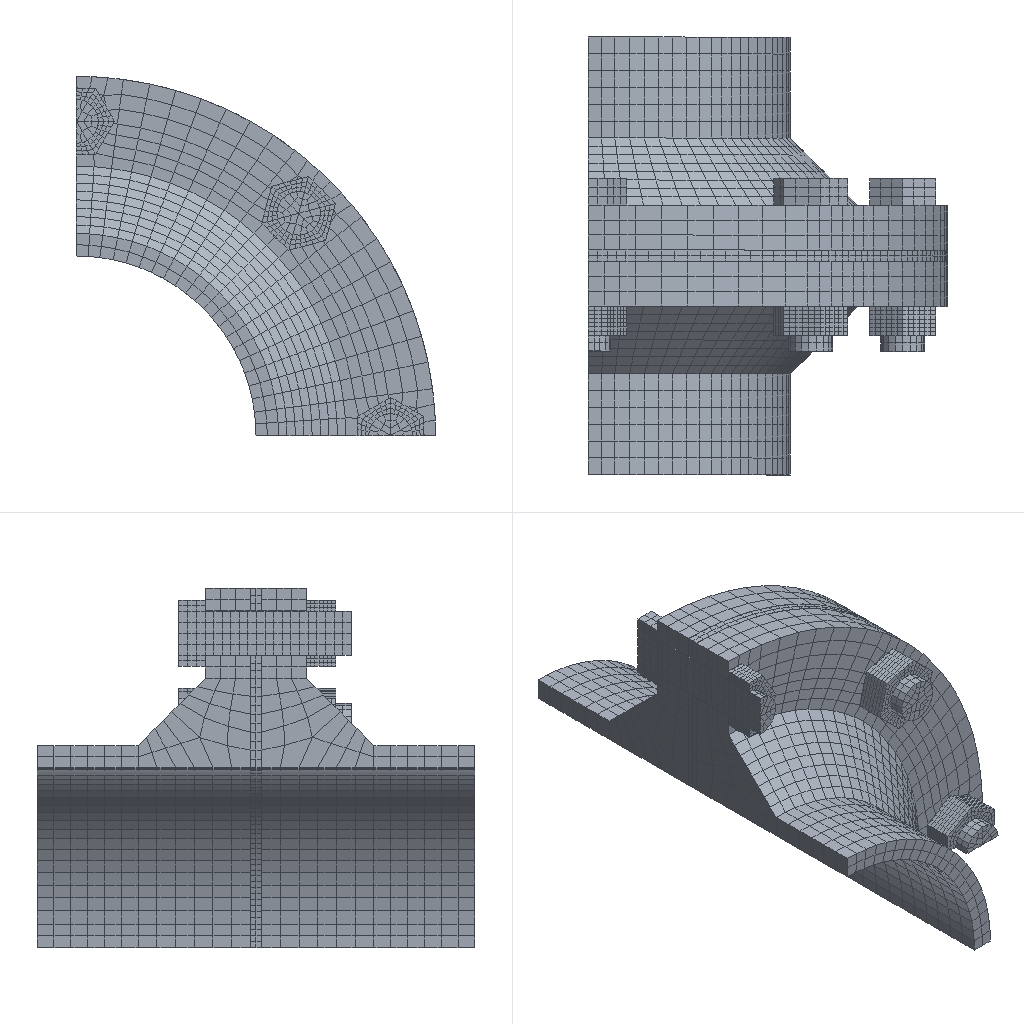Simulation study | abaqus
Set-up summary:
category,name,step,type,value,unit,region
solver,abaqus,,Abaqus/CAE 2024
units,mm-mN-s-kg (kPa) or mm-kg-s,,inferred,E=1.4935e+07 density=
analysis,Tighten bolts,,static,nlgeom=True; time_period=1
mesh,nodes,,,11472
mesh,elements,,,7304
element_type,C3D8R,,,5496
element_type,C3D8H,,,1808
material,brass,,E,1.4935e+07
material,brass,,nu,0.3
material,brass,,yield,28000
material,brass,,behaviors,plastic
material,rubber,,behaviors,hyperelastic
material,steel,,E,3e+07
material,steel,,nu,0.3
material,steel,,yield,52000
material,steel,,behaviors,plastic
section,steel,,solid section,,,all
section,brass,,solid section,,,all
section,rubber,,solid section,,,all
section,steel,,solid section,,,all
section,steel,,solid section,,,all
section,steel,,solid section,,,all
load,Load-1,Tighten bolts,concentrated force,"200 [dir=(1, 0, 0)]",,_Load-1_blrn_
load,Load-2,Tighten bolts,concentrated force,"100 [dir=(1, 0, 0)]",,_Load-2_blrn_
load,Load-3,Tighten bolts,concentrated force,"100 [dir=(1, 0, 0)]",,_Load-3_blrn_
bc,Bottom,Tighten bolts,fixed,[dofs=y],,Bottom
bc,Csymm-x,Tighten bolts,fixed,[dofs=x],,Csymm-x
bc,Csymm-z,Tighten bolts,fixed,[dofs=z],,Csymm-z
contact,CP-1-HalfBolt-1-HalfNut-1,initial,tie,,,CP-1-HalfNut-1 / CP-1-HalfBolt-1
contact,CP-2-Bolt-1-nut-1,initial,tie,,,CP-2-nut-1 / CP-2-Bolt-1
contact,CP-3-HalfBolt-2-HalfNut-2,initial,tie,,,CP-3-HalfNut-2 / CP-3-HalfBolt-2
contact,CP-1-botFlange-Gasket-1,initial,contact pair surface to surface,interaction=Friction-0p4; friction=0.4; behavior=hard,,CP-1-Gasket-1 / CP-1-botFlange
contact,CP-2-botFlange-Bolt-1,initial,contact pair surface to surface,interaction=Friction-0p1; friction=0.1; behavior=hard,,CP-3-Bolt-1 / CP-2-botFlange
contact,CP-3-botFlange-nut-1,initial,contact pair surface to surface,interaction=Friction-0p1; friction=0.1; behavior=hard,,CP-3-nut-1 / CP-3-botFlange
contact,CP-4-botFlange-HalfBolt-1,initial,contact pair surface to surface,interaction=Friction-0p1; friction=0.1; behavior=hard,,CP-4-HalfBolt-1 / CP-4-botFlange
contact,CP-5-botFlange-HalfNut-1,initial,contact pair surface to surface,interaction=Friction-0p1; friction=0.1; behavior=hard,,CP-5-HalfNut-1 / CP-5-botFlange
contact,CP-6-botFlange-HalfBolt-2,initial,contact pair surface to surface,interaction=Friction-0p1; friction=0.1; behavior=hard,,CP-6-HalfBolt-2 / CP-6-botFlange
contact,CP-7-botFlange-HalfNut-2,initial,contact pair surface to surface,interaction=Friction-0p1; friction=0.1; behavior=hard,,CP-7-HalfNut-2 / CP-7-botFlange
contact,CP-8-topFlange-Gasket-1,initial,contact pair surface to surface,interaction=Friction-0p4; friction=0.4; behavior=hard,,CP-8-Gasket-1 / CP-8-topFlange
contact,CP-9-topFlange-Bolt-1,initial,contact pair surface to surface,interaction=Friction-0p1; friction=0.1; behavior=hard,,CP-9-Bolt-1 / CP-9-topFlange
contact,CP-10-topFlange-Bolt-1,initial,contact pair surface to surface,interaction=Friction-0p1; friction=0.1; behavior=hard,,CP-10-Bolt-1 / CP-10-topFlange
contact,CP-11-topFlange-HalfBolt-1,initial,contact pair surface to surface,interaction=Friction-0p1; friction=0.1; behavior=hard,,CP-11-HalfBolt-1 / CP-11-topFlange
contact,CP-12-topFlange-HalfBolt-1,initial,contact pair surface to surface,interaction=Friction-0p1; friction=0.1; behavior=hard,,CP-12-HalfBolt-1 / CP-12-topFlange
contact,CP-13-topFlange-HalfBolt-2,initial,contact pair surface to surface,interaction=Friction-0p1; friction=0.1; behavior=hard,,CP-13-HalfBolt-2 / CP-13-topFlange
contact,CP-14-topFlange-HalfBolt-2,initial,contact pair surface to surface,interaction=Friction-0p1; friction=0.1; behavior=hard,,CP-14-HalfBolt-2 / CP-14-topFlange
contact,CP-15-Bolt-1-Gasket-1,initial,contact pair surface to surface,interaction=Friction-0p4; friction=0.4; behavior=hard,,CP-15-Gasket-1 / CP-15-Bolt-1
contact,CP-16-HalfBolt-1-Gasket-1,initial,contact pair surface to surface,interaction=Friction-0p4; friction=0.4; behavior=hard,,CP-16-Gasket-1 / CP-16-HalfBolt-1
contact,CP-17-HalfBolt-2-Gasket-1,initial,contact pair surface to surface,interaction=Friction-0p4; friction=0.4; behavior=hard,,CP-17-Gasket-1 / CP-17-HalfBolt-2
Abaqus input file, long lists of numbers shortened, first 294 of 1956 lines:
*Heading
** Job name: deck Model name: Model-1
** Generated by: Abaqus/CAE 2024
*Preprint, echo=NO, model=NO, history=NO, contact=NO
**
** PARTS
**
*Part, name=bolt
*Node
      1, -1.5239944e-10,  0.85, -4.02707534e-10
      2,  0.1225,  0.85,  0.2122
** (982 more lines like these left out)
*Element, type=C3D8R
 1, 318,  55, 294, 770,  41,   1,  42, 292
 2, 770, 294, 295, 763, 292,  42,  43, 293
** (706 more lines like these left out)
*Nset, nset=all, generate
   1,  984,    1
*Elset, elset=all, generate
   1,  708,    1
*Elset, elset=_boltLoad_S2, internal
   1,   2,  13,  19,  20,  66,  67,  78,  84,  85, 131, 132, 143, 149, 150, 196
 202, 203, 214, 215, 261, 262, 273, 279, 280, 504
*Elset, elset=_boltLoad_S4, internal
 482, 489
*Elset, elset=_boltLoad_S3, internal
 490, 497
*Surface, type=ELEMENT, name=boltLoad
_boltLoad_S2, S2
_boltLoad_S4, S4
_boltLoad_S3, S3
** Section: bolt
*Solid Section, elset=all, material=steel
1.,
*End Part
**
*Part, name=flange
*Node
      1,           2.,  0.5244,           0.
      2,   1.983,  0.5244,   0.2611
** (1981 more lines like these left out)
*Element, type=C3D8R
 1,  634,  635, 1561, 1560,   93,   94,  629,  628
 2,  635,  636, 1562, 1561,   94,   95,  630,  629
** (1256 more lines like these left out)
*Nset, nset=all, generate
    1,  1983,     1
*Elset, elset=all, generate
    1,  1258,     1
** Section: flange
*Solid Section, elset=all, material=brass
1.,
*End Part
**
*Part, name=gasket
*Node
      1,   3.47,  0.4568,        0.125
      2,   3.47,  0.4568,           0.
** (2965 more lines like these left out)
*Element, type=C3D8H
 1,  716,   74,  706, 2319,   71,    1,   73,  704
 2, 2319,  706,  707, 2316,  704,   73,   72,  705
** (1806 more lines like these left out)
*Nset, nset=all, generate
    1,  2967,     1
*Elset, elset=all, generate
    1,  1808,     1
** Section: gasket
*Solid Section, elset=all, material=rubber
1.,
*End Part
**
*Part, name=halfBolt
*Node
      1, -6.66499911e-11,   1.225, -1.78729587e-10
      2, -0.2122,   1.225, -0.1225
** (590 more lines like these left out)
*Element, type=C3D8R
 1, 221,  37, 218, 480,  35,   1,  36, 217
 2, 222,  38, 219, 479, 221,  37, 218, 480
** (378 more lines like these left out)
*Nset, nset=all, generate
   1,  592,    1
*Elset, elset=all, generate
   1,  380,    1
*Elset, elset=_boltLoad_S4, internal
  37,  51, 130, 195, 202
*Elset, elset=_boltLoad_S3, internal
  38, 131, 175, 182
*Elset, elset=_boltLoad_S2, internal
 138, 203, 250, 251, 262, 263, 274
*Surface, type=ELEMENT, name=boltLoad
_boltLoad_S4, S4
_boltLoad_S3, S3
_boltLoad_S2, S2
** Section: bolt
*Solid Section, elset=all, material=steel
1.,
*End Part
**
*Part, name=halfNut
*Node
      1, -0.2125, -0.3681,  0.325
      2, -0.425,           0.,  0.325
** (606 more lines like these left out)
*Element, type=C3D8R
  1,  67, 241, 441, 217,   1,  21, 157,  42
  2, 241, 242, 442, 441,  21,  22, 158, 157
** (376 more lines like these left out)
*Nset, nset=all, generate
   1,  608,    1
*Elset, elset=all, generate
   1,  378,    1
** Section: bolt
*Solid Section, elset=all, material=steel
1.,
*End Part
**
*Part, name=nut
*Node
      1,  0.425,           0.,  0.325
      2,  0.2125, -0.3681,  0.325
** (1150 more lines like these left out)
*Element, type=C3D8R
  1,  72, 325, 793, 301,   1,  25, 241,  46
  2, 325, 326, 794, 793,  25,  26, 242, 241
** (754 more lines like these left out)
*Nset, nset=all, generate
    1,  1152,     1
*Elset, elset=all, generate
   1,  756,    1
** Section: bolt
*Solid Section, elset=all, material=steel
1.,
*End Part
**
**
** ASSEMBLY
**
*Assembly, name=Assembly
**
*Instance, name=botFlange, part=flange
*End Instance
**
*Instance, name=topFlange, part=flange
          0.,     3.674,           0.
          0.,     3.674,           0., 0.7071,     3.674, 0.7071,         180.
*End Instance
**
*Instance, name=Gasket-1, part=gasket
          0.,     1.774, -8.99865743746394e-13
          0.,     1.774, -8.99865743746394e-13, 0.5774, 2.352, 0.5774,         240.
*End Instance
**
*Instance, name=Bolt-1, part=bolt
2.475,     1.174, 2.475
2.475,     1.174, 2.475, 2.475, 0.1744, 2.475, 15.
*End Instance
**
*Instance, name=nut-1, part=nut
2.475,     1.274, 2.475
2.475,     1.274, 2.475, 3.458, 1.145, 2.604, 90.976
*End Instance
**
*Instance, name=HalfBolt-1, part=halfBolt
          0.,     1.174,          3.5
          0.,     1.174,          3.5,           0.,     0.1744,          3.5, 60.
*End Instance
**
*Instance, name=HalfNut-1, part=halfNut
1.63712270681787e-11,     1.274,          3.5
1.63712270681787e-11,     1.274,          3.5, 1.8118469336612e-11, 1.981, 2.793, 180.
*End Instance
**
*Instance, name=HalfBolt-2, part=halfBolt
         3.5,     1.174, 2.45732323378434e-11
         3.5,     1.174, 2.45732323378434e-11,          3.5, 2.174, 2.45732323378434e-11, 210.
*End Instance
**
*Instance, name=HalfNut-2, part=halfNut
         3.5,     1.274, 1.63713487211226e-11
         3.5,     1.274, 1.63713487211226e-11, 4.077, 1.852, -0.5774,         120.
*End Instance
**
*Nset, nset=Bottom, instance=botFlange
   31,   32,   33,   34,   35,   36,   37,   38,   39,   40,   41,   42,   64,   65,  281,  282
  283,  284,  305,  306,  307,  308,  309,  310,  311,  312,  313,  314,  315,  316,  317,  328
** (3 more lines like these left out)
*Elset, elset=Bottom, instance=botFlange
 461, 462, 463, 464, 535, 536, 537, 538, 539, 540, 541, 542, 543, 544, 545, 546
 547, 548, 569, 570, 571, 572, 593, 594, 595, 596, 667, 668, 669, 670, 671, 672
** (1 more lines like these left out)
*Nset, nset=Csymm-x, instance=botFlange
   43,   44,   45,   46,   47,   52,   53,   54,   55,   58,   59,   64,   65,  379,  380,  381
  382,  383,  384,  385,  386,  387,  388,  392,  393,  394,  395,  396,  397,  398,  399,  400
** (3 more lines like these left out)
*Nset, nset=Csymm-x, instance=topFlange
    1,    4,    5,    9,   10,   33,   34,   86,   87,   88,   89,   90,   91,   92,   93,   94
   95,   96,   98,  110,  111,  112,  113,  115,  116,  117,  118,  119,  120,  121,  133,  134
** (3 more lines like these left out)
*Nset, nset=Csymm-x, instance=HalfNut-1
   9,  10,  11,  12,  17,  18,  19,  20,  73,  74,  75,  76,  77,  78,  83,  84
  85,  86,  87,  88,  93,  94,  95,  96, 133, 134, 135, 136, 137, 138, 143, 144
** (2 more lines like these left out)
*Nset, nset=Csymm-x, instance=Gasket-1
    7,    8,    9,   10,   13,   14,   15,   16,   24,   25,  100,  101,  102,  103,  104,  105
  128,  129,  130,  131,  137,  138,  245,  246,  247,  248,  249,  250,  251,  252,  253,  266
** (2 more lines like these left out)
*Nset, nset=Csymm-x, instance=HalfBolt-1
   1,   2,   4,   5,   7,   8,  10,  12,  17,  18,  19,  20,  21,  25,  26,  27
  35,  37,  38,  39,  41,  42,  43,  47,  51,  52,  53,  54,  55,  56,  57,  58
** (6 more lines like these left out)
*Elset, elset=Csymm-x, instance=botFlange
 689, 690, 691, 692, 693, 694, 695, 696, 711, 712, 713, 714, 715, 716, 717, 718
 719, 720, 721, 722, 723, 724, 746, 747, 748, 749, 750, 751, 759, 760, 761, 774
** (1 more lines like these left out)
*Elset, elset=Csymm-x, instance=topFlange
    1,    2,    3,    4,   11,   12,   13,   14,   15,   16,   33,   34,   35,   36,   37,   38
   39,   40,   41,   42,   43,   44,  443,  444,  447,  448,  451,  452,  455,  456,  459,  460
** (1 more lines like these left out)
*Elset, elset=Csymm-x, instance=HalfNut-1
 127, 128, 129, 130, 131, 132, 133, 148, 149, 150, 151, 152, 153, 154, 169, 170
 171, 172, 173, 174, 175, 316, 317, 318, 319, 320, 321, 322, 337, 338, 339, 340
** (1 more lines like these left out)
*Elset, elset=Csymm-x, instance=Gasket-1
  28,  29,  30,  34,  36,  38,  64,  65,  66,  76,  79,  80, 393, 394, 395, 396
 397, 398, 399, 400, 401, 402, 433, 434, 435, 436, 437, 438, 439, 440, 441, 442
*Elset, elset=Csymm-x, instance=HalfBolt-1
   1,   2,   3,   4,   7,   8,   9,  10,  13,  14,  15,  16,  17,  18,  19,  20
  21,  22,  23,  24,  31,  32,  33,  34,  35,  36,  37,  38,  39,  40,  41,  42
** (4 more lines like these left out)
*Nset, nset=Csymm-z, instance=botFlange
    1,    4,    5,    9,   10,   33,   34,   86,   87,   88,   89,   90,   91,   92,   93,   94
   95,   96,   98,  110,  111,  112,  113,  115,  116,  117,  118,  119,  120,  121,  133,  134
** (3 more lines like these left out)
*Nset, nset=Csymm-z, instance=topFlange
   43,   44,   45,   46,   47,   52,   53,   54,   55,   58,   59,   64,   65,  379,  380,  381
  382,  383,  384,  385,  386,  387,  388,  392,  393,  394,  395,  396,  397,  398,  399,  400
** (3 more lines like these left out)
*Nset, nset=Csymm-z, instance=HalfBolt-2
   1,   2,   4,   5,   7,   8,  10,  12,  17,  18,  19,  20,  21,  25,  26,  27
  35,  37,  38,  39,  41,  42,  43,  47,  51,  52,  53,  54,  55,  56,  57,  58
** (6 more lines like these left out)
*Nset, nset=Csymm-z, instance=HalfNut-2
   9,  10,  11,  12,  17,  18,  19,  20,  73,  74,  75,  76,  77,  78,  83,  84
  85,  86,  87,  88,  93,  94,  95,  96, 133, 134, 135, 136, 137, 138, 143, 144
** (2 more lines like these left out)
*Nset, nset=Csymm-z, instance=Gasket-1
   59,   60,   61,   62,   65,   66,   67,   68,   69,   70,  630,  631,  632,  633,  634,  635
  636,  637,  638,  639,  640,  641,  642,  643,  644,  645,  646,  647,  648,  649,  677,  678
** (2 more lines like these left out)
*Elset, elset=Csymm-z, instance=botFlange
    1,    2,    3,    4,   11,   12,   13,   14,   15,   16,   33,   34,   35,   36,   37,   38
   39,   40,   41,   42,   43,   44,  443,  444,  447,  448,  451,  452,  455,  456,  459,  460
** (1 more lines like these left out)
*Elset, elset=Csymm-z, instance=topFlange
 689, 690, 691, 692, 693, 694, 695, 696, 711, 712, 713, 714, 715, 716, 717, 718
 719, 720, 721, 722, 723, 724, 746, 747, 748, 749, 750, 751, 759, 760, 761, 774
** (1 more lines like these left out)
*Elset, elset=Csymm-z, instance=HalfBolt-2
   1,   2,   3,   4,   7,   8,   9,  10,  13,  14,  15,  16,  17,  18,  19,  20
  21,  22,  23,  24,  31,  32,  33,  34,  35,  36,  37,  38,  39,  40,  41,  42
** (4 more lines like these left out)
*Elset, elset=Csymm-z, instance=HalfNut-2
 127, 128, 129, 130, 131, 132, 133, 148, 149, 150, 151, 152, 153, 154, 169, 170
 171, 172, 173, 174, 175, 316, 317, 318, 319, 320, 321, 322, 337, 338, 339, 340
** (1 more lines like these left out)
*Elset, elset=Csymm-z, instance=Gasket-1
 1647, 1648, 1649, 1650, 1651, 1652, 1653, 1654, 1655, 1656, 1657, 1658, 1659, 1660, 1661, 1662
 1663, 1664, 1665, 1666, 1735, 1736, 1761, 1764, 1767, 1770, 1771, 1772, 1775, 1776, 1779, 1781
*Elset, elset=_CP-1-Gasket-1_S5, internal, instance=Gasket-1
 228, 229, 230, 231, 232, 238, 239, 240, 241, 242, 248, 249, 250, 251, 252, 258
 259, 260, 261, 262, 268, 269, 270, 271, 272, 278, 279, 280, 281, 282, 288, 289
** (3 more lines like these left out)
*Elset, elset=_CP-1-Gasket-1_S2, internal, instance=Gasket-1
   27,   28,   29,   30,   31,   32,   74,   75,   76,   77,   78,   79,   80,   81,   82,  363
  364,  365,  366,  367,  368,  369,  370,  371,  372,  373,  374,  375,  376,  377,  378,  379
** (3 more lines like these left out)
*Elset, elset=_CP-1-Gasket-1_S4, internal, instance=Gasket-1
   13,   14,   15,   49,   50,   51,   52,   84,   86,   88,   90,   92,   94,   96,   98,  100
  102,  104,  106,  108,  110,  112,  114,  116,  118,  120,  122,  124,  126,  128,  130,  132
** (36 more lines like these left out)
*Elset, elset=_CP-1-Gasket-1_S3, internal, instance=Gasket-1
    7,    8,    9,   10,   11,   12,   19,   20,   21,   22,   53,   54,   55,   56,   57,   58
   71,   72,   73,  818,  819,  820,  835,  836,  837,  838,  839,  840,  857,  858,  859,  860
** (9 more lines like these left out)
*Surface, type=ELEMENT, name=CP-1-Gasket-1
_CP-1-Gasket-1_S5, S5
_CP-1-Gasket-1_S2, S2
_CP-1-Gasket-1_S4, S4
_CP-1-Gasket-1_S3, S3
*Elset, elset=_CP-1-HalfBolt-1_S4, internal, instance=HalfBolt-1
   5,   6,  19,  20,  21,  22,  23,  24,  38,  39,  40,  41,  42,  43,  44,  56
  57, 118, 119, 120, 121, 122, 123, 157, 158, 159, 160, 161, 162, 163, 164, 165
Last 389 lines:
__CP-16-HalfBolt-1-Gasket-1_msm_1_S3, S3
*Elset, elset=__CP-16-HalfBolt-1-Gasket-1_msm_2_S3, internal, instance=HalfBolt-1
 54, 55, 58, 59, 62, 63
*Elset, elset=__CP-16-HalfBolt-1-Gasket-1_msm_2_S4, internal, instance=HalfBolt-1
 56, 57
*Surface, type=ELEMENT, name=_CP-16-HalfBolt-1-Gasket-1_msm_2, internal
__CP-16-HalfBolt-1-Gasket-1_msm_2_S3, S3
__CP-16-HalfBolt-1-Gasket-1_msm_2_S4, S4
*Elset, elset=__CP-16-HalfBolt-1-Gasket-1_msm_3_S3, internal, instance=HalfBolt-1
 214, 215, 216, 217, 224, 225, 226, 227, 228, 229
*Elset, elset=__CP-16-HalfBolt-1-Gasket-1_msm_3_S4, internal, instance=HalfBolt-1
 218, 219
*Surface, type=ELEMENT, name=_CP-16-HalfBolt-1-Gasket-1_msm_3, internal
__CP-16-HalfBolt-1-Gasket-1_msm_3_S3, S3
__CP-16-HalfBolt-1-Gasket-1_msm_3_S4, S4
*Elset, elset=__CP-16-HalfBolt-1-Gasket-1_msm_4_S4, internal, instance=HalfBolt-1
 262, 263, 264, 265, 266, 267, 268, 269, 270, 271, 272, 273, 294, 295, 296, 297
 298, 299, 300, 301, 302, 303, 304, 305, 306, 307
*Elset, elset=__CP-16-HalfBolt-1-Gasket-1_msm_4_S3, internal, instance=HalfBolt-1
 274, 275, 276, 277, 278, 279, 308, 309, 310, 311, 312, 313, 314
*Surface, type=ELEMENT, name=_CP-16-HalfBolt-1-Gasket-1_msm_4, internal
__CP-16-HalfBolt-1-Gasket-1_msm_4_S4, S4
__CP-16-HalfBolt-1-Gasket-1_msm_4_S3, S3
*Elset, elset=__CP-16-HalfBolt-1-Gasket-1_msm_5_S3, internal, instance=HalfBolt-1
 106, 107, 108, 109, 110, 111, 124, 125, 126, 127, 128, 129, 130, 138, 139, 140
 141, 142, 143, 144
*Elset, elset=__CP-16-HalfBolt-1-Gasket-1_msm_5_S4, internal, instance=HalfBolt-1, generate
 118,  123,    1
*Surface, type=ELEMENT, name=_CP-16-HalfBolt-1-Gasket-1_msm_5, internal
__CP-16-HalfBolt-1-Gasket-1_msm_5_S3, S3
__CP-16-HalfBolt-1-Gasket-1_msm_5_S4, S4
*Elset, elset=__CP-16-HalfBolt-1-Gasket-1_msm_6_S3, internal, instance=HalfBolt-1
  3,  4,  7,  8, 11, 12
*Elset, elset=__CP-16-HalfBolt-1-Gasket-1_msm_6_S4, internal, instance=HalfBolt-1
 5, 6
*Surface, type=ELEMENT, name=_CP-16-HalfBolt-1-Gasket-1_msm_6, internal
__CP-16-HalfBolt-1-Gasket-1_msm_6_S3, S3
__CP-16-HalfBolt-1-Gasket-1_msm_6_S4, S4
*Elset, elset=__CP-16-HalfBolt-1-Gasket-1_msm_7_S4, internal, instance=HalfBolt-1
 157, 158, 159, 160, 161, 162, 163, 164, 165, 166, 167, 168, 175, 176, 177, 178
 179, 180, 181, 182, 183, 184, 185, 186, 187, 188, 203, 204, 205, 206, 207, 208
** (1 more lines like these left out)
*Elset, elset=__CP-16-HalfBolt-1-Gasket-1_msm_7_S3, internal, instance=HalfBolt-1, generate
 169,  174,    1
*Surface, type=ELEMENT, name=_CP-16-HalfBolt-1-Gasket-1_msm_7, internal
__CP-16-HalfBolt-1-Gasket-1_msm_7_S4, S4
__CP-16-HalfBolt-1-Gasket-1_msm_7_S3, S3
*Elset, elset=__CP-16-HalfBolt-1-Gasket-1_msm_8_S3, internal, instance=HalfBolt-1
 234, 235, 242, 243, 244, 245, 246, 247, 248, 249
*Elset, elset=__CP-16-HalfBolt-1-Gasket-1_msm_8_S4, internal, instance=HalfBolt-1
 236, 237
*Surface, type=ELEMENT, name=_CP-16-HalfBolt-1-Gasket-1_msm_8, internal
__CP-16-HalfBolt-1-Gasket-1_msm_8_S3, S3
__CP-16-HalfBolt-1-Gasket-1_msm_8_S4, S4
*Elset, elset=__CP-16-HalfBolt-1-Gasket-1_ssm_1_S3, internal, instance=Gasket-1
 13, 14, 15, 27, 28
*Elset, elset=__CP-16-HalfBolt-1-Gasket-1_ssm_1_S4, internal, instance=Gasket-1, generate
 16,  18,   1
*Elset, elset=__CP-16-HalfBolt-1-Gasket-1_ssm_1_S2, internal, instance=Gasket-1
 33, 34
*Surface, type=ELEMENT, name=_CP-16-HalfBolt-1-Gasket-1_ssm_1, internal
__CP-16-HalfBolt-1-Gasket-1_ssm_1_S3, S3
__CP-16-HalfBolt-1-Gasket-1_ssm_1_S4, S4
__CP-16-HalfBolt-1-Gasket-1_ssm_1_S2, S2
*Elset, elset=__CP-16-HalfBolt-1-Gasket-1_ssm_2_S4, internal, instance=Gasket-1
 59, 60, 61, 71, 72, 73, 80, 81, 82
*Elset, elset=__CP-16-HalfBolt-1-Gasket-1_ssm_2_S3, internal, instance=Gasket-1, generate
 62,  64,   1
*Surface, type=ELEMENT, name=_CP-16-HalfBolt-1-Gasket-1_ssm_2, internal
__CP-16-HalfBolt-1-Gasket-1_ssm_2_S4, S4
__CP-16-HalfBolt-1-Gasket-1_ssm_2_S3, S3
*Elset, elset=__CP-17-HalfBolt-2-Gasket-1_msm_1_S4, internal, instance=HalfBolt-2
 19, 20, 21, 22, 23, 24, 38, 39, 40, 41, 42, 43, 44
*Elset, elset=__CP-17-HalfBolt-2-Gasket-1_msm_1_S3, internal, instance=HalfBolt-2
 25, 26, 27, 28, 29, 30, 45, 46, 47, 48, 49, 50, 51
*Surface, type=ELEMENT, name=_CP-17-HalfBolt-2-Gasket-1_msm_1, internal
__CP-17-HalfBolt-2-Gasket-1_msm_1_S4, S4
__CP-17-HalfBolt-2-Gasket-1_msm_1_S3, S3
*Elset, elset=__CP-17-HalfBolt-2-Gasket-1_msm_2_S3, internal, instance=HalfBolt-2
 54, 55, 58, 59, 62, 63
*Elset, elset=__CP-17-HalfBolt-2-Gasket-1_msm_2_S4, internal, instance=HalfBolt-2
 56, 57
*Surface, type=ELEMENT, name=_CP-17-HalfBolt-2-Gasket-1_msm_2, internal
__CP-17-HalfBolt-2-Gasket-1_msm_2_S3, S3
__CP-17-HalfBolt-2-Gasket-1_msm_2_S4, S4
*Elset, elset=__CP-17-HalfBolt-2-Gasket-1_msm_3_S3, internal, instance=HalfBolt-2
 214, 215, 216, 217, 224, 225, 226, 227, 228, 229
*Elset, elset=__CP-17-HalfBolt-2-Gasket-1_msm_3_S4, internal, instance=HalfBolt-2
 218, 219
*Surface, type=ELEMENT, name=_CP-17-HalfBolt-2-Gasket-1_msm_3, internal
__CP-17-HalfBolt-2-Gasket-1_msm_3_S3, S3
__CP-17-HalfBolt-2-Gasket-1_msm_3_S4, S4
*Elset, elset=__CP-17-HalfBolt-2-Gasket-1_msm_4_S4, internal, instance=HalfBolt-2
 262, 263, 264, 265, 266, 267, 268, 269, 270, 271, 272, 273, 294, 295, 296, 297
 298, 299, 300, 301, 302, 303, 304, 305, 306, 307
*Elset, elset=__CP-17-HalfBolt-2-Gasket-1_msm_4_S3, internal, instance=HalfBolt-2
 274, 275, 276, 277, 278, 279, 308, 309, 310, 311, 312, 313, 314
*Surface, type=ELEMENT, name=_CP-17-HalfBolt-2-Gasket-1_msm_4, internal
__CP-17-HalfBolt-2-Gasket-1_msm_4_S4, S4
__CP-17-HalfBolt-2-Gasket-1_msm_4_S3, S3
*Elset, elset=__CP-17-HalfBolt-2-Gasket-1_msm_5_S3, internal, instance=HalfBolt-2
 106, 107, 108, 109, 110, 111, 124, 125, 126, 127, 128, 129, 130, 138, 139, 140
 141, 142, 143, 144
*Elset, elset=__CP-17-HalfBolt-2-Gasket-1_msm_5_S4, internal, instance=HalfBolt-2, generate
 118,  123,    1
*Surface, type=ELEMENT, name=_CP-17-HalfBolt-2-Gasket-1_msm_5, internal
__CP-17-HalfBolt-2-Gasket-1_msm_5_S3, S3
__CP-17-HalfBolt-2-Gasket-1_msm_5_S4, S4
*Elset, elset=__CP-17-HalfBolt-2-Gasket-1_msm_6_S3, internal, instance=HalfBolt-2
  3,  4,  7,  8, 11, 12
*Elset, elset=__CP-17-HalfBolt-2-Gasket-1_msm_6_S4, internal, instance=HalfBolt-2
 5, 6
*Surface, type=ELEMENT, name=_CP-17-HalfBolt-2-Gasket-1_msm_6, internal
__CP-17-HalfBolt-2-Gasket-1_msm_6_S3, S3
__CP-17-HalfBolt-2-Gasket-1_msm_6_S4, S4
*Elset, elset=__CP-17-HalfBolt-2-Gasket-1_msm_7_S4, internal, instance=HalfBolt-2
 157, 158, 159, 160, 161, 162, 163, 164, 165, 166, 167, 168, 175, 176, 177, 178
 179, 180, 181, 182, 183, 184, 185, 186, 187, 188, 203, 204, 205, 206, 207, 208
** (1 more lines like these left out)
*Elset, elset=__CP-17-HalfBolt-2-Gasket-1_msm_7_S3, internal, instance=HalfBolt-2, generate
 169,  174,    1
*Surface, type=ELEMENT, name=_CP-17-HalfBolt-2-Gasket-1_msm_7, internal
__CP-17-HalfBolt-2-Gasket-1_msm_7_S4, S4
__CP-17-HalfBolt-2-Gasket-1_msm_7_S3, S3
*Elset, elset=__CP-17-HalfBolt-2-Gasket-1_msm_8_S3, internal, instance=HalfBolt-2
 234, 235, 242, 243, 244, 245, 246, 247, 248, 249
*Elset, elset=__CP-17-HalfBolt-2-Gasket-1_msm_8_S4, internal, instance=HalfBolt-2
 236, 237
*Surface, type=ELEMENT, name=_CP-17-HalfBolt-2-Gasket-1_msm_8, internal
__CP-17-HalfBolt-2-Gasket-1_msm_8_S3, S3
__CP-17-HalfBolt-2-Gasket-1_msm_8_S4, S4
*Elset, elset=__CP-17-HalfBolt-2-Gasket-1_ssm_1_S2, internal, instance=Gasket-1, generate
 1727,  1738,     1
*Surface, type=ELEMENT, name=_CP-17-HalfBolt-2-Gasket-1_ssm_1, internal
__CP-17-HalfBolt-2-Gasket-1_ssm_1_S2, S2
*Elset, elset=__CP-17-HalfBolt-2-Gasket-1_ssm_2_S4, internal, instance=Gasket-1
 1779, 1780, 1806, 1807, 1808
*Elset, elset=__CP-17-HalfBolt-2-Gasket-1_ssm_2_S3, internal, instance=Gasket-1
 1781, 1782, 1803, 1804, 1805
*Surface, type=ELEMENT, name=_CP-17-HalfBolt-2-Gasket-1_ssm_2, internal
__CP-17-HalfBolt-2-Gasket-1_ssm_2_S4, S4
__CP-17-HalfBolt-2-Gasket-1_ssm_2_S3, S3
*End Assembly
**
** MATERIALS
**
*Material, name=brass
*Elastic
 1.4935e+07, 0.3
*Plastic
28000.,  0.
30000., 0.1
*Material, name=rubber
*Hyperelastic, mooney-rivlin
556.,    139., 2.8e-05
*Material, name=steel
*Elastic
 3e+07, 0.3
*Plastic
52000.,  0.
65000., 0.1
**
** INTERACTION PROPERTIES
**
*Surface Interaction, name=Friction-0p1
1.,
*Friction, slip tolerance=0.005
 0.1,
*Surface Behavior, penalty
*Surface Interaction, name=Friction-0p4
1.,
*Friction, slip tolerance=0.005
 0.4,
*Surface Behavior, penalty
*Surface Smoothing, name=CP-2-botFlange-Bolt-1
, _CP-2-botFlange-Bolt-1_msm_1, CIRCUMFERENTIAL, 2.475, 1.774, 2.475, 2.475, 0.7744, 2.475
, _CP-2-botFlange-Bolt-1_msm_2, CIRCUMFERENTIAL, 2.475, 1.774, 2.475, 2.475, 0.7744, 2.475
, _CP-2-botFlange-Bolt-1_msm_3, CIRCUMFERENTIAL, 2.475, 1.774, 2.475, 2.475, 0.7744, 2.475
, _CP-2-botFlange-Bolt-1_msm_4, CIRCUMFERENTIAL, 2.475, 1.774, 2.475, 2.475, 0.7744, 2.475
_CP-2-botFlange-Bolt-1_ssm_1, , CIRCUMFERENTIAL, 2.475, 1.587, 2.475, 2.475, 0.5869, 2.475
_CP-2-botFlange-Bolt-1_ssm_2, , CIRCUMFERENTIAL, 2.475, 1.587, 2.475, 2.475, 0.5869, 2.475
_CP-2-botFlange-Bolt-1_ssm_3, , CIRCUMFERENTIAL, 2.475, 1.587, 2.475, 2.475, 0.5869, 2.475
_CP-2-botFlange-Bolt-1_ssm_4, , CIRCUMFERENTIAL, 2.475, 1.587, 2.475, 2.475, 0.5869, 2.475
_CP-2-botFlange-Bolt-1_ssm_5, , CIRCUMFERENTIAL, 2.475, 1.587, 2.475, 2.475, 0.5869, 2.475
_CP-2-botFlange-Bolt-1_ssm_6, , CIRCUMFERENTIAL, 2.475, 1.587, 2.475, 2.475, 0.5869, 2.475
_CP-2-botFlange-Bolt-1_ssm_7, , CIRCUMFERENTIAL, 2.475, 1.587, 2.475, 2.475, 0.5869, 2.475
_CP-2-botFlange-Bolt-1_ssm_8, , CIRCUMFERENTIAL, 2.475, 1.587, 2.475, 2.475, 0.5869, 2.475
_CP-2-botFlange-Bolt-1_ssm_9, , CIRCUMFERENTIAL, 2.475, 1.587, 2.475, 2.475, 0.5869, 2.475
_CP-2-botFlange-Bolt-1_ssm_10, , CIRCUMFERENTIAL, 2.475, 1.587, 2.475, 2.475, 0.5869, 2.475
_CP-2-botFlange-Bolt-1_ssm_11, , CIRCUMFERENTIAL, 2.475, 1.587, 2.475, 2.475, 0.5869, 2.475
_CP-2-botFlange-Bolt-1_ssm_12, , CIRCUMFERENTIAL, 2.475, 1.587, 2.475, 2.475, 0.5869, 2.475
*Surface Smoothing, name=CP-4-botFlange-HalfBolt-1
, _CP-4-botFlange-HalfBolt-1_msm_1, CIRCUMFERENTIAL, 4.9738e-14, 1.774, 3.5, 4.9738e-14, 0.7744, 3.5
, _CP-4-botFlange-HalfBolt-1_msm_2, CIRCUMFERENTIAL, 4.9738e-14, 1.774, 3.5, 4.9738e-14, 0.7744, 3.5
_CP-4-botFlange-HalfBolt-1_ssm_1, , CIRCUMFERENTIAL, 0., 1.587, 3.5, 0., 0.5869, 3.5
_CP-4-botFlange-HalfBolt-1_ssm_2, , CIRCUMFERENTIAL, 0., 1.587, 3.5, 0., 0.5869, 3.5
_CP-4-botFlange-HalfBolt-1_ssm_3, , CIRCUMFERENTIAL, 0., 1.587, 3.5, 0., 0.5869, 3.5
_CP-4-botFlange-HalfBolt-1_ssm_4, , CIRCUMFERENTIAL, 0., 1.587, 3.5, 0., 0.5869, 3.5
_CP-4-botFlange-HalfBolt-1_ssm_5, , CIRCUMFERENTIAL, 0., 1.587, 3.5, 0., 0.5869, 3.5
_CP-4-botFlange-HalfBolt-1_ssm_6, , CIRCUMFERENTIAL, 0., 1.587, 3.5, 0., 0.5869, 3.5
_CP-4-botFlange-HalfBolt-1_ssm_7, , CIRCUMFERENTIAL, 0., 1.587, 3.5, 0., 0.5869, 3.5
_CP-4-botFlange-HalfBolt-1_ssm_8, , CIRCUMFERENTIAL, 0., 1.587, 3.5, 0., 0.5869, 3.5
*Surface Smoothing, name=CP-6-botFlange-HalfBolt-2
, _CP-6-botFlange-HalfBolt-2_msm_1, CIRCUMFERENTIAL, 3.5, 1.774, 4.9738e-14, 3.5, 0.7744, 4.9738e-14
, _CP-6-botFlange-HalfBolt-2_msm_2, CIRCUMFERENTIAL, 3.5, 1.774, 4.9738e-14, 3.5, 0.7744, 4.9738e-14
_CP-6-botFlange-HalfBolt-2_ssm_1, , CIRCUMFERENTIAL, 3.5, 1.587, 2.45732e-11, 3.5, 0.5869, 2.45732e-11
_CP-6-botFlange-HalfBolt-2_ssm_2, , CIRCUMFERENTIAL, 3.5, 1.587, 2.45732e-11, 3.5, 0.5869, 2.45732e-11
_CP-6-botFlange-HalfBolt-2_ssm_3, , CIRCUMFERENTIAL, 3.5, 1.587, 2.45732e-11, 3.5, 0.5869, 2.45732e-11
_CP-6-botFlange-HalfBolt-2_ssm_4, , CIRCUMFERENTIAL, 3.5, 1.587, 2.45732e-11, 3.5, 0.5869, 2.45732e-11
_CP-6-botFlange-HalfBolt-2_ssm_5, , CIRCUMFERENTIAL, 3.5, 1.587, 2.45732e-11, 3.5, 0.5869, 2.45732e-11
_CP-6-botFlange-HalfBolt-2_ssm_6, , CIRCUMFERENTIAL, 3.5, 1.587, 2.45732e-11, 3.5, 0.5869, 2.45732e-11
_CP-6-botFlange-HalfBolt-2_ssm_7, , CIRCUMFERENTIAL, 3.5, 1.587, 2.45732e-11, 3.5, 0.5869, 2.45732e-11
_CP-6-botFlange-HalfBolt-2_ssm_8, , CIRCUMFERENTIAL, 3.5, 1.587, 2.45732e-11, 3.5, 0.5869, 2.45732e-11
*Surface Smoothing, name=CP-9-topFlange-Bolt-1
, _CP-9-topFlange-Bolt-1_msm_1, CIRCUMFERENTIAL, 2.475, 1.899, 2.475, 2.475, 2.899, 2.475
, _CP-9-topFlange-Bolt-1_msm_2, CIRCUMFERENTIAL, 2.475, 1.899, 2.475, 2.475, 2.899, 2.475
, _CP-9-topFlange-Bolt-1_msm_3, CIRCUMFERENTIAL, 2.475, 1.899, 2.475, 2.475, 2.899, 2.475
, _CP-9-topFlange-Bolt-1_msm_4, CIRCUMFERENTIAL, 2.475, 1.899, 2.475, 2.475, 2.899, 2.475
_CP-9-topFlange-Bolt-1_ssm_1, , CIRCUMFERENTIAL, 2.475, 1.587, 2.475, 2.475, 0.5869, 2.475
_CP-9-topFlange-Bolt-1_ssm_2, , CIRCUMFERENTIAL, 2.475, 1.587, 2.475, 2.475, 0.5869, 2.475
_CP-9-topFlange-Bolt-1_ssm_3, , CIRCUMFERENTIAL, 2.475, 1.587, 2.475, 2.475, 0.5869, 2.475
_CP-9-topFlange-Bolt-1_ssm_4, , CIRCUMFERENTIAL, 2.475, 1.587, 2.475, 2.475, 0.5869, 2.475
_CP-9-topFlange-Bolt-1_ssm_5, , CIRCUMFERENTIAL, 2.475, 1.587, 2.475, 2.475, 0.5869, 2.475
_CP-9-topFlange-Bolt-1_ssm_6, , CIRCUMFERENTIAL, 2.475, 1.587, 2.475, 2.475, 0.5869, 2.475
_CP-9-topFlange-Bolt-1_ssm_7, , CIRCUMFERENTIAL, 2.475, 1.587, 2.475, 2.475, 0.5869, 2.475
_CP-9-topFlange-Bolt-1_ssm_8, , CIRCUMFERENTIAL, 2.475, 1.587, 2.475, 2.475, 0.5869, 2.475
_CP-9-topFlange-Bolt-1_ssm_9, , CIRCUMFERENTIAL, 2.475, 1.587, 2.475, 2.475, 0.5869, 2.475
_CP-9-topFlange-Bolt-1_ssm_10, , CIRCUMFERENTIAL, 2.475, 1.587, 2.475, 2.475, 0.5869, 2.475
_CP-9-topFlange-Bolt-1_ssm_11, , CIRCUMFERENTIAL, 2.475, 1.587, 2.475, 2.475, 0.5869, 2.475
_CP-9-topFlange-Bolt-1_ssm_12, , CIRCUMFERENTIAL, 2.475, 1.587, 2.475, 2.475, 0.5869, 2.475
*Surface Smoothing, name=CP-12-topFlange-HalfBolt-1
, _CP-12-topFlange-HalfBolt-1_msm_1, CIRCUMFERENTIAL, 5.02402e-14, 1.899, 3.5, 5.01536e-14, 2.899, 3.5
, _CP-12-topFlange-HalfBolt-1_msm_2, CIRCUMFERENTIAL, 5.02402e-14, 1.899, 3.5, 5.01536e-14, 2.899, 3.5
_CP-12-topFlange-HalfBolt-1_ssm_1, , CIRCUMFERENTIAL, 0., 1.587, 3.5, 0., 0.5869, 3.5
_CP-12-topFlange-HalfBolt-1_ssm_2, , CIRCUMFERENTIAL, 0., 1.587, 3.5, 0., 0.5869, 3.5
_CP-12-topFlange-HalfBolt-1_ssm_3, , CIRCUMFERENTIAL, 0., 1.587, 3.5, 0., 0.5869, 3.5
_CP-12-topFlange-HalfBolt-1_ssm_4, , CIRCUMFERENTIAL, 0., 1.587, 3.5, 0., 0.5869, 3.5
_CP-12-topFlange-HalfBolt-1_ssm_5, , CIRCUMFERENTIAL, 0., 1.587, 3.5, 0., 0.5869, 3.5
_CP-12-topFlange-HalfBolt-1_ssm_6, , CIRCUMFERENTIAL, 0., 1.587, 3.5, 0., 0.5869, 3.5
_CP-12-topFlange-HalfBolt-1_ssm_7, , CIRCUMFERENTIAL, 0., 1.587, 3.5, 0., 0.5869, 3.5
_CP-12-topFlange-HalfBolt-1_ssm_8, , CIRCUMFERENTIAL, 0., 1.587, 3.5, 0., 0.5869, 3.5
*Surface Smoothing, name=CP-14-topFlange-HalfBolt-2
, _CP-14-topFlange-HalfBolt-2_msm_1, CIRCUMFERENTIAL, 3.5, 1.899, 5.10974e-14, 3.5, 2.899, 5.10108e-14
, _CP-14-topFlange-HalfBolt-2_msm_2, CIRCUMFERENTIAL, 3.5, 1.899, 5.10974e-14, 3.5, 2.899, 5.10108e-14
_CP-14-topFlange-HalfBolt-2_ssm_1, , CIRCUMFERENTIAL, 3.5, 1.587, 2.45732e-11, 3.5, 0.5869, 2.45732e-11
_CP-14-topFlange-HalfBolt-2_ssm_2, , CIRCUMFERENTIAL, 3.5, 1.587, 2.45732e-11, 3.5, 0.5869, 2.45732e-11
_CP-14-topFlange-HalfBolt-2_ssm_3, , CIRCUMFERENTIAL, 3.5, 1.587, 2.45732e-11, 3.5, 0.5869, 2.45732e-11
_CP-14-topFlange-HalfBolt-2_ssm_4, , CIRCUMFERENTIAL, 3.5, 1.587, 2.45732e-11, 3.5, 0.5869, 2.45732e-11
_CP-14-topFlange-HalfBolt-2_ssm_5, , CIRCUMFERENTIAL, 3.5, 1.587, 2.45732e-11, 3.5, 0.5869, 2.45732e-11
_CP-14-topFlange-HalfBolt-2_ssm_6, , CIRCUMFERENTIAL, 3.5, 1.587, 2.45732e-11, 3.5, 0.5869, 2.45732e-11
_CP-14-topFlange-HalfBolt-2_ssm_7, , CIRCUMFERENTIAL, 3.5, 1.587, 2.45732e-11, 3.5, 0.5869, 2.45732e-11
_CP-14-topFlange-HalfBolt-2_ssm_8, , CIRCUMFERENTIAL, 3.5, 1.587, 2.45732e-11, 3.5, 0.5869, 2.45732e-11
*Surface Smoothing, name=CP-15-Bolt-1-Gasket-1
, _CP-15-Bolt-1-Gasket-1_msm_1, CIRCUMFERENTIAL, 2.475, 1.587, 2.475, 2.475, 0.5869, 2.475
, _CP-15-Bolt-1-Gasket-1_msm_2, CIRCUMFERENTIAL, 2.475, 1.587, 2.475, 2.475, 0.5869, 2.475
, _CP-15-Bolt-1-Gasket-1_msm_3, CIRCUMFERENTIAL, 2.475, 1.587, 2.475, 2.475, 0.5869, 2.475
, _CP-15-Bolt-1-Gasket-1_msm_4, CIRCUMFERENTIAL, 2.475, 1.587, 2.475, 2.475, 0.5869, 2.475
, _CP-15-Bolt-1-Gasket-1_msm_5, CIRCUMFERENTIAL, 2.475, 1.587, 2.475, 2.475, 0.5869, 2.475
, _CP-15-Bolt-1-Gasket-1_msm_6, CIRCUMFERENTIAL, 2.475, 1.587, 2.475, 2.475, 0.5869, 2.475
, _CP-15-Bolt-1-Gasket-1_msm_7, CIRCUMFERENTIAL, 2.475, 1.587, 2.475, 2.475, 0.5869, 2.475
, _CP-15-Bolt-1-Gasket-1_msm_8, CIRCUMFERENTIAL, 2.475, 1.587, 2.475, 2.475, 0.5869, 2.475
, _CP-15-Bolt-1-Gasket-1_msm_9, CIRCUMFERENTIAL, 2.475, 1.587, 2.475, 2.475, 0.5869, 2.475
, _CP-15-Bolt-1-Gasket-1_msm_10, CIRCUMFERENTIAL, 2.475, 1.587, 2.475, 2.475, 0.5869, 2.475
, _CP-15-Bolt-1-Gasket-1_msm_11, CIRCUMFERENTIAL, 2.475, 1.587, 2.475, 2.475, 0.5869, 2.475
, _CP-15-Bolt-1-Gasket-1_msm_12, CIRCUMFERENTIAL, 2.475, 1.587, 2.475, 2.475, 0.5869, 2.475
_CP-15-Bolt-1-Gasket-1_ssm_1, , CIRCUMFERENTIAL, 2.475, 1.774, 2.475, 2.475, 2.774, 2.475
_CP-15-Bolt-1-Gasket-1_ssm_2, , CIRCUMFERENTIAL, 2.475, 1.774, 2.475, 2.475, 2.774, 2.475
_CP-15-Bolt-1-Gasket-1_ssm_3, , CIRCUMFERENTIAL, 2.475, 1.774, 2.475, 2.475, 2.774, 2.475
_CP-15-Bolt-1-Gasket-1_ssm_4, , CIRCUMFERENTIAL, 2.475, 1.774, 2.475, 2.475, 2.774, 2.475
*Surface Smoothing, name=CP-16-HalfBolt-1-Gasket-1
, _CP-16-HalfBolt-1-Gasket-1_msm_1, CIRCUMFERENTIAL, 0., 1.587, 3.5, 0., 0.5869, 3.5
, _CP-16-HalfBolt-1-Gasket-1_msm_2, CIRCUMFERENTIAL, 0., 1.587, 3.5, 0., 0.5869, 3.5
, _CP-16-HalfBolt-1-Gasket-1_msm_3, CIRCUMFERENTIAL, 0., 1.587, 3.5, 0., 0.5869, 3.5
, _CP-16-HalfBolt-1-Gasket-1_msm_4, CIRCUMFERENTIAL, 0., 1.587, 3.5, 0., 0.5869, 3.5
, _CP-16-HalfBolt-1-Gasket-1_msm_5, CIRCUMFERENTIAL, 0., 1.587, 3.5, 0., 0.5869, 3.5
, _CP-16-HalfBolt-1-Gasket-1_msm_6, CIRCUMFERENTIAL, 0., 1.587, 3.5, 0., 0.5869, 3.5
, _CP-16-HalfBolt-1-Gasket-1_msm_7, CIRCUMFERENTIAL, 0., 1.587, 3.5, 0., 0.5869, 3.5
, _CP-16-HalfBolt-1-Gasket-1_msm_8, CIRCUMFERENTIAL, 0., 1.587, 3.5, 0., 0.5869, 3.5
_CP-16-HalfBolt-1-Gasket-1_ssm_1, , CIRCUMFERENTIAL, -8.87714e-17, 1.774, 3.5, -1.0115e-16, 2.774, 3.5
_CP-16-HalfBolt-1-Gasket-1_ssm_2, , CIRCUMFERENTIAL, -8.87714e-17, 1.774, 3.5, -1.0115e-16, 2.774, 3.5
*Surface Smoothing, name=CP-17-HalfBolt-2-Gasket-1
, _CP-17-HalfBolt-2-Gasket-1_msm_1, CIRCUMFERENTIAL, 3.5, 1.587, 2.45732e-11, 3.5, 0.5869, 2.45732e-11
, _CP-17-HalfBolt-2-Gasket-1_msm_2, CIRCUMFERENTIAL, 3.5, 1.587, 2.45732e-11, 3.5, 0.5869, 2.45732e-11
, _CP-17-HalfBolt-2-Gasket-1_msm_3, CIRCUMFERENTIAL, 3.5, 1.587, 2.45732e-11, 3.5, 0.5869, 2.45732e-11
, _CP-17-HalfBolt-2-Gasket-1_msm_4, CIRCUMFERENTIAL, 3.5, 1.587, 2.45732e-11, 3.5, 0.5869, 2.45732e-11
, _CP-17-HalfBolt-2-Gasket-1_msm_5, CIRCUMFERENTIAL, 3.5, 1.587, 2.45732e-11, 3.5, 0.5869, 2.45732e-11
, _CP-17-HalfBolt-2-Gasket-1_msm_6, CIRCUMFERENTIAL, 3.5, 1.587, 2.45732e-11, 3.5, 0.5869, 2.45732e-11
, _CP-17-HalfBolt-2-Gasket-1_msm_7, CIRCUMFERENTIAL, 3.5, 1.587, 2.45732e-11, 3.5, 0.5869, 2.45732e-11
, _CP-17-HalfBolt-2-Gasket-1_msm_8, CIRCUMFERENTIAL, 3.5, 1.587, 2.45732e-11, 3.5, 0.5869, 2.45732e-11
_CP-17-HalfBolt-2-Gasket-1_ssm_1, , CIRCUMFERENTIAL, 3.5, 1.774, -8.99777e-13, 3.5, 2.774, -8.99864e-13
_CP-17-HalfBolt-2-Gasket-1_ssm_2, , CIRCUMFERENTIAL, 3.5, 1.774, -8.99777e-13, 3.5, 2.774, -8.99864e-13
**
** INTERACTIONS
**
** Interaction: CP-1-botFlange-Gasket-1
*Contact Pair, interaction=Friction-0p4, small sliding, type=SURFACE TO SURFACE, adjust=0.01
CP-1-Gasket-1, CP-1-botFlange
** Interaction: CP-2-botFlange-Bolt-1
*Contact Pair, interaction=Friction-0p1, small sliding, type=SURFACE TO SURFACE, geometric correction=CP-2-botFlange-Bolt-1
CP-3-Bolt-1, CP-2-botFlange
** Interaction: CP-3-botFlange-nut-1
*Contact Pair, interaction=Friction-0p1, small sliding, type=SURFACE TO SURFACE, adjust=0.01
CP-3-nut-1, CP-3-botFlange
** Interaction: CP-4-botFlange-HalfBolt-1
*Contact Pair, interaction=Friction-0p1, small sliding, type=SURFACE TO SURFACE, geometric correction=CP-4-botFlange-HalfBolt-1
CP-4-HalfBolt-1, CP-4-botFlange
** Interaction: CP-5-botFlange-HalfNut-1
*Contact Pair, interaction=Friction-0p1, small sliding, type=SURFACE TO SURFACE, adjust=0.01
CP-5-HalfNut-1, CP-5-botFlange
** Interaction: CP-6-botFlange-HalfBolt-2
*Contact Pair, interaction=Friction-0p1, small sliding, type=SURFACE TO SURFACE, geometric correction=CP-6-botFlange-HalfBolt-2
CP-6-HalfBolt-2, CP-6-botFlange
** Interaction: CP-7-botFlange-HalfNut-2
*Contact Pair, interaction=Friction-0p1, small sliding, type=SURFACE TO SURFACE, adjust=0.01
CP-7-HalfNut-2, CP-7-botFlange
** Interaction: CP-8-topFlange-Gasket-1
*Contact Pair, interaction=Friction-0p4, small sliding, type=SURFACE TO SURFACE, adjust=0.01
CP-8-Gasket-1, CP-8-topFlange
** Interaction: CP-9-topFlange-Bolt-1
*Contact Pair, interaction=Friction-0p1, small sliding, type=SURFACE TO SURFACE, geometric correction=CP-9-topFlange-Bolt-1
CP-9-Bolt-1, CP-9-topFlange
** Interaction: CP-10-topFlange-Bolt-1
*Contact Pair, interaction=Friction-0p1, small sliding, type=SURFACE TO SURFACE, adjust=0.01
CP-10-Bolt-1, CP-10-topFlange
** Interaction: CP-11-topFlange-HalfBolt-1
*Contact Pair, interaction=Friction-0p1, small sliding, type=SURFACE TO SURFACE, adjust=0.01
CP-11-HalfBolt-1, CP-11-topFlange
** Interaction: CP-12-topFlange-HalfBolt-1
*Contact Pair, interaction=Friction-0p1, small sliding, type=SURFACE TO SURFACE, geometric correction=CP-12-topFlange-HalfBolt-1
CP-12-HalfBolt-1, CP-12-topFlange
** Interaction: CP-13-topFlange-HalfBolt-2
*Contact Pair, interaction=Friction-0p1, small sliding, type=SURFACE TO SURFACE, adjust=0.01
CP-13-HalfBolt-2, CP-13-topFlange
** Interaction: CP-14-topFlange-HalfBolt-2
*Contact Pair, interaction=Friction-0p1, small sliding, type=SURFACE TO SURFACE, geometric correction=CP-14-topFlange-HalfBolt-2
CP-14-HalfBolt-2, CP-14-topFlange
** Interaction: CP-15-Bolt-1-Gasket-1
*Contact Pair, interaction=Friction-0p4, small sliding, type=SURFACE TO SURFACE, geometric correction=CP-15-Bolt-1-Gasket-1
CP-15-Gasket-1, CP-15-Bolt-1
** Interaction: CP-16-HalfBolt-1-Gasket-1
*Contact Pair, interaction=Friction-0p4, small sliding, type=SURFACE TO SURFACE, geometric correction=CP-16-HalfBolt-1-Gasket-1
CP-16-Gasket-1, CP-16-HalfBolt-1
** Interaction: CP-17-HalfBolt-2-Gasket-1
*Contact Pair, interaction=Friction-0p4, small sliding, type=SURFACE TO SURFACE, geometric correction=CP-17-HalfBolt-2-Gasket-1
CP-17-Gasket-1, CP-17-HalfBolt-2
** ----------------------------------------------------------------
**
** STEP: Tighten bolts
**
*Step, name="Tighten bolts", nlgeom=YES
*Static
0.25, 1., 1e-05, 1.
**
** BOUNDARY CONDITIONS
**
** Name: Bottom Type: Displacement/Rotation
*Boundary
Bottom, 2, 2
** Name: Csymm-x Type: Displacement/Rotation
*Boundary
Csymm-x, 1, 1
** Name: Csymm-z Type: Displacement/Rotation
*Boundary
Csymm-z, 3, 3
**
** LOADS
**
** Name: Load-1   Type: Bolt load
*Cload
_Load-1_blrn_, 1, 200.
** Name: Load-2   Type: Bolt load
*Cload
_Load-2_blrn_, 1, 100.
** Name: Load-3   Type: Bolt load
*Cload
_Load-3_blrn_, 1, 100.
**
** OUTPUT REQUESTS
**
*Restart, write, frequency=0
**
** FIELD OUTPUT: F-Output-1
**
*Output, field, variable=PRESELECT
**
** HISTORY OUTPUT: H-Output-1
**
*Output, history, variable=PRESELECT
*End Step
Results summary:
result,odb.job_status,,,JOB_STATUS_COMPLETED_SUCCESSFULLY,"consistent, unstated (Abaqus has no unit system)"
result,steps[0].procedure,Tighten bolts,,*STATIC,"consistent, unstated (Abaqus has no unit system)"
result,steps[0].time_period,Tighten bolts,,1,"consistent, unstated (Abaqus has no unit system)"
result,steps[0].n_frames,Tighten bolts,,5,"consistent, unstated (Abaqus has no unit system)"
result,steps[0].last_frame.id,Tighten bolts,,4,"consistent, unstated (Abaqus has no unit system)"
result,steps[0].last_frame.value,Tighten bolts,,1,"consistent, unstated (Abaqus has no unit system)"
result,steps[0].last_frame.description,Tighten bolts,,Increment      4: Step Time =    1.000,"consistent, unstated (Abaqus has no unit system)"
result,steps[0].completed,Tighten bolts,,True,"consistent, unstated (Abaqus has no unit system)"
result,steps[0].max_U_magnitude,Tighten bolts,,0.001021,"consistent, unstated (Abaqus has no unit system)"
result,steps[0].max_S_mises,Tighten bolts,,2128.23,"consistent, unstated (Abaqus has no unit system)"
result,steps[0].RF_sum[1],Tighten bolts,,-1.57952e-06,"consistent, unstated (Abaqus has no unit system)"
result,steps[0].RF_sum[2],Tighten bolts,,-1.95578e-07,"consistent, unstated (Abaqus has no unit system)"
result,steps[0].RF_sum[3],Tighten bolts,,1.19209e-07,"consistent, unstated (Abaqus has no unit system)"